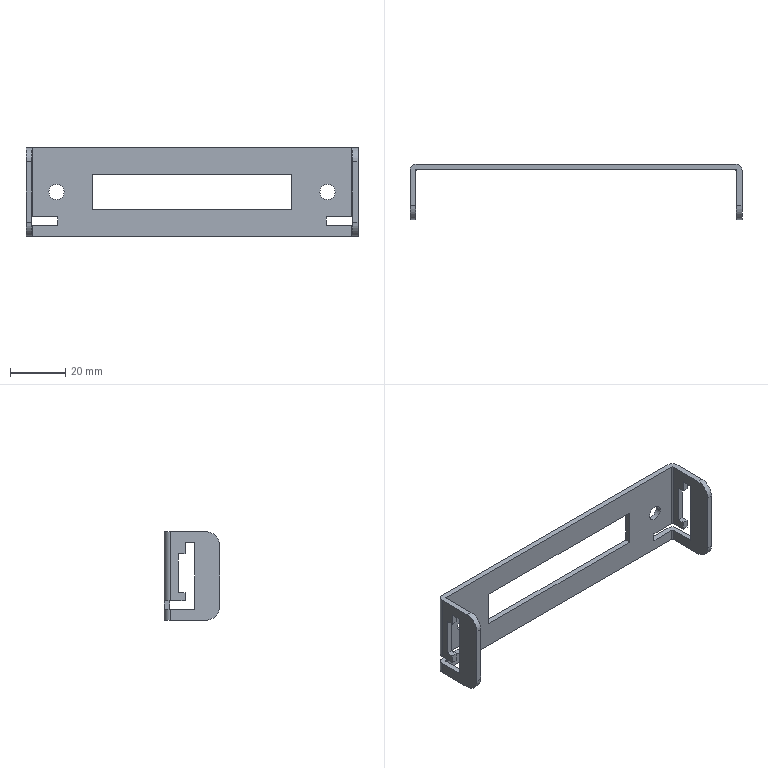Part | STEP file | Pull rod connecting plate | 1 solid | 50 faces | box 120 x 20 x 32 mm | volume 7229 mm3 | plane 34 | cylinder 16 | commonest cylinder face diameters 0.6 x4 4.6 x4 5.5 x4 10 x4